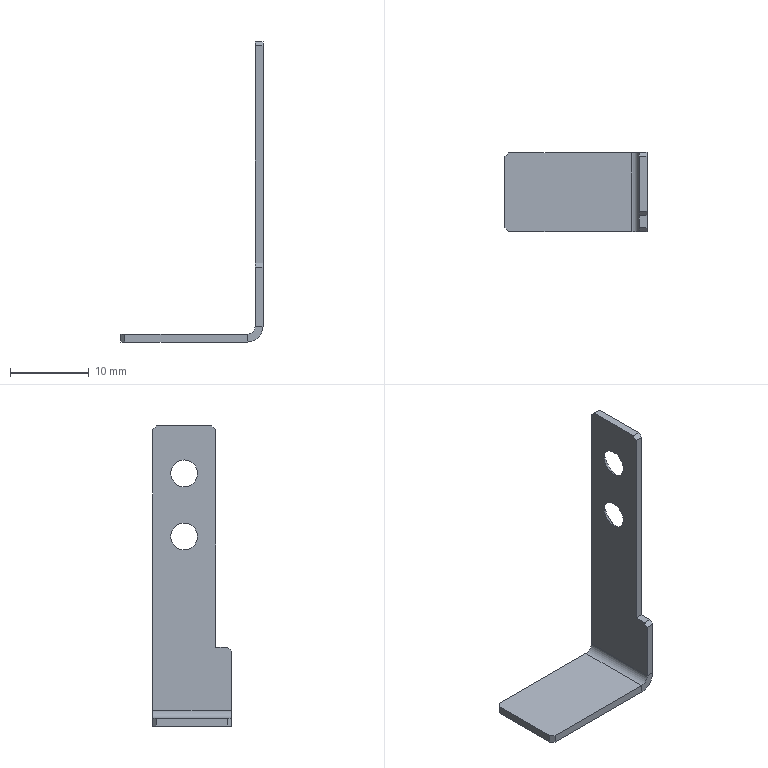Part | NX | features BREP 1 | 1 solid | 25 faces | box 18 x 10 x 38 mm | volume 456.003 mm3 | plane 19 | cone 4 | cylinder 2 | commonest cylinder face diameters 2 x1 4 x1
STEP:
#1=CARTESIAN_POINT('',(-1.,4.5,19.));
#2=VERTEX_POINT('',#1);
#3=CARTESIAN_POINT('',(-1.,5.,18.5));
#4=VERTEX_POINT('',#3);
#5=CARTESIAN_POINT('',(-1.,5.,18.5));
#6=DIRECTION('',(0.,0.7071,-0.7071));
#7=VECTOR('',#6,1000.);
#8=LINE('',#5,#7);
#9=EDGE_CURVE('',#2,#4,#8,.T.);
#10=ORIENTED_EDGE('',*,*,#9,.F.);
#11=CARTESIAN_POINT('',(0.,4.5,19.));
#12=VERTEX_POINT('',#11);
#13=CARTESIAN_POINT('',(-1.,4.5,19.));
#14=DIRECTION('',(-1.,0.,0.));
#15=VECTOR('',#14,1000.);
#16=LINE('',#13,#15);
#17=EDGE_CURVE('',#12,#2,#16,.T.);
#18=ORIENTED_EDGE('',*,*,#17,.F.);
#19=CARTESIAN_POINT('',(0.,5.,18.5));
#20=VERTEX_POINT('',#19);
#21=CARTESIAN_POINT('',(0.,11.75,11.75));
#22=DIRECTION('',(0.,-0.7071,0.7071));
#23=VECTOR('',#22,1000.);
#24=LINE('',#21,#23);
#25=EDGE_CURVE('',#20,#12,#24,.T.);
#26=ORIENTED_EDGE('',*,*,#25,.F.);
#27=CARTESIAN_POINT('',(-1.,5.,18.5));
#28=DIRECTION('',(1.,0.,0.));
#29=VECTOR('',#28,1000.);
#30=LINE('',#27,#29);
#31=EDGE_CURVE('',#4,#20,#30,.T.);
#32=ORIENTED_EDGE('',*,*,#31,.F.);
#33=EDGE_LOOP('',(#10,#18,#26,#32));
#34=FACE_BOUND('',#33,.T.);
#35=CARTESIAN_POINT('',(-1.,5.,18.5));
#36=DIRECTION('',(0.,-0.7071,-0.7071));
#37=DIRECTION('',(1.,0.,0.));
#38=AXIS2_PLACEMENT_3D('',#35,#36,#37);
#39=PLANE('',#38);
#40=ADVANCED_FACE('',(#34),#39,.F.);
#41=CARTESIAN_POINT('',(0.,-2.5,19.));
#42=VERTEX_POINT('',#41);
#43=CARTESIAN_POINT('',(0.,-3.,18.5));
#44=VERTEX_POINT('',#43);
#45=CARTESIAN_POINT('',(0.,-10.75,10.75));
#46=DIRECTION('',(0.,-0.7071,-0.7071));
#47=VECTOR('',#46,1000.);
#48=LINE('',#45,#47);
#49=EDGE_CURVE('',#42,#44,#48,.T.);
#50=ORIENTED_EDGE('',*,*,#49,.F.);
#51=CARTESIAN_POINT('',(-1.,-2.5,19.));
#52=VERTEX_POINT('',#51);
#53=CARTESIAN_POINT('',(0.,-2.5,19.));
#54=DIRECTION('',(1.,0.,0.));
#55=VECTOR('',#54,1000.);
#56=LINE('',#53,#55);
#57=EDGE_CURVE('',#52,#42,#56,.T.);
#58=ORIENTED_EDGE('',*,*,#57,.F.);
#59=CARTESIAN_POINT('',(-1.,-3.,18.5));
#60=VERTEX_POINT('',#59);
#61=CARTESIAN_POINT('',(-1.,-3.,18.5));
#62=DIRECTION('',(0.,0.7071,0.7071));
#63=VECTOR('',#62,1000.);
#64=LINE('',#61,#63);
#65=EDGE_CURVE('',#60,#52,#64,.T.);
#66=ORIENTED_EDGE('',*,*,#65,.F.);
#67=CARTESIAN_POINT('',(-1.,-3.,18.5));
#68=DIRECTION('',(-1.,0.,0.));
#69=VECTOR('',#68,1000.);
#70=LINE('',#67,#69);
#71=EDGE_CURVE('',#44,#60,#70,.T.);
#72=ORIENTED_EDGE('',*,*,#71,.F.);
#73=EDGE_LOOP('',(#50,#58,#66,#72));
#74=FACE_BOUND('',#73,.T.);
#75=CARTESIAN_POINT('',(-18.,-3.,18.5));
#76=DIRECTION('',(0.,-0.7071,0.7071));
#77=DIRECTION('',(1.,0.,0.));
#78=AXIS2_PLACEMENT_3D('',#75,#76,#77);
#79=PLANE('',#78);
#80=ADVANCED_FACE('',(#74),#79,.T.);
#81=CARTESIAN_POINT('',(-1.,-5.,-9.5));
#82=VERTEX_POINT('',#81);
#83=CARTESIAN_POINT('',(-1.,-4.5,-9.));
#84=VERTEX_POINT('',#83);
#85=CARTESIAN_POINT('',(-1.,-4.5,-9.));
#86=DIRECTION('',(0.,0.7071,0.7071));
#87=VECTOR('',#86,1000.);
#88=LINE('',#85,#87);
#89=EDGE_CURVE('',#82,#84,#88,.T.);
#90=ORIENTED_EDGE('',*,*,#89,.F.);
#91=CARTESIAN_POINT('',(0.,-5.,-9.5));
#92=VERTEX_POINT('',#91);
#93=CARTESIAN_POINT('',(-1.,-5.,-9.5));
#94=DIRECTION('',(-1.,0.,0.));
#95=VECTOR('',#94,1000.);
#96=LINE('',#93,#95);
#97=EDGE_CURVE('',#92,#82,#96,.T.);
#98=ORIENTED_EDGE('',*,*,#97,.F.);
#99=CARTESIAN_POINT('',(0.,-4.5,-9.));
#100=VERTEX_POINT('',#99);
#101=CARTESIAN_POINT('',(0.,2.25,-2.25));
#102=DIRECTION('',(0.,-0.7071,-0.7071));
#103=VECTOR('',#102,1000.);
#104=LINE('',#101,#103);
#105=EDGE_CURVE('',#100,#92,#104,.T.);
#106=ORIENTED_EDGE('',*,*,#105,.F.);
#107=CARTESIAN_POINT('',(0.,-4.5,-9.));
#108=DIRECTION('',(1.,0.,0.));
#109=VECTOR('',#108,1000.);
#110=LINE('',#107,#109);
#111=EDGE_CURVE('',#84,#100,#110,.T.);
#112=ORIENTED_EDGE('',*,*,#111,.F.);
#113=EDGE_LOOP('',(#90,#98,#106,#112));
#114=FACE_BOUND('',#113,.T.);
#115=CARTESIAN_POINT('',(-18.,-4.5,-9.));
#116=DIRECTION('',(0.,-0.7071,0.7071));
#117=DIRECTION('',(-1.,0.,0.));
#118=AXIS2_PLACEMENT_3D('',#115,#116,#117);
#119=PLANE('',#118);
#120=ADVANCED_FACE('',(#114),#119,.T.);
#121=CARTESIAN_POINT('',(-17.5,-5.,-19.));
#122=VERTEX_POINT('',#121);
#123=CARTESIAN_POINT('',(-18.,-4.5,-19.));
#124=VERTEX_POINT('',#123);
#125=CARTESIAN_POINT('',(-18.,-4.5,-19.));
#126=DIRECTION('',(-0.7071,0.7071,0.));
#127=VECTOR('',#126,1000.);
#128=LINE('',#125,#127);
#129=EDGE_CURVE('',#122,#124,#128,.T.);
#130=ORIENTED_EDGE('',*,*,#129,.F.);
#131=CARTESIAN_POINT('',(-17.5,-5.,-18.));
#132=VERTEX_POINT('',#131);
#133=CARTESIAN_POINT('',(-17.5,-5.,-19.));
#134=DIRECTION('',(0.,0.,-1.));
#135=VECTOR('',#134,1000.);
#136=LINE('',#133,#135);
#137=EDGE_CURVE('',#132,#122,#136,.T.);
#138=ORIENTED_EDGE('',*,*,#137,.F.);
#139=CARTESIAN_POINT('',(-18.,-4.5,-18.));
#140=VERTEX_POINT('',#139);
#141=CARTESIAN_POINT('',(-11.25,-11.25,-18.));
#142=DIRECTION('',(0.7071,-0.7071,0.));
#143=VECTOR('',#142,1000.);
#144=LINE('',#141,#143);
#145=EDGE_CURVE('',#140,#132,#144,.T.);
#146=ORIENTED_EDGE('',*,*,#145,.F.);
#147=CARTESIAN_POINT('',(-18.,-4.5,-19.));
#148=DIRECTION('',(0.,0.,1.));
#149=VECTOR('',#148,1000.);
#150=LINE('',#147,#149);
#151=EDGE_CURVE('',#124,#140,#150,.T.);
#152=ORIENTED_EDGE('',*,*,#151,.F.);
#153=EDGE_LOOP('',(#130,#138,#146,#152));
#154=FACE_BOUND('',#153,.T.);
#155=CARTESIAN_POINT('',(-18.,-4.5,-19.));
#156=DIRECTION('',(0.7071,0.7071,0.));
#157=DIRECTION('',(0.,0.,1.));
#158=AXIS2_PLACEMENT_3D('',#155,#156,#157);
#159=PLANE('',#158);
#160=ADVANCED_FACE('',(#154),#159,.F.);
#161=CARTESIAN_POINT('',(-18.,4.5,-19.));
#162=VERTEX_POINT('',#161);
#163=CARTESIAN_POINT('',(-17.5,5.,-19.));
#164=VERTEX_POINT('',#163);
#165=CARTESIAN_POINT('',(-17.5,5.,-19.));
#166=DIRECTION('',(0.7071,0.7071,0.));
#167=VECTOR('',#166,1000.);
#168=LINE('',#165,#167);
#169=EDGE_CURVE('',#162,#164,#168,.T.);
#170=ORIENTED_EDGE('',*,*,#169,.F.);
#171=CARTESIAN_POINT('',(-18.,4.5,-18.));
#172=VERTEX_POINT('',#171);
#173=CARTESIAN_POINT('',(-18.,4.5,-19.));
#174=DIRECTION('',(0.,0.,-1.));
#175=VECTOR('',#174,1000.);
#176=LINE('',#173,#175);
#177=EDGE_CURVE('',#172,#162,#176,.T.);
#178=ORIENTED_EDGE('',*,*,#177,.F.);
#179=CARTESIAN_POINT('',(-17.5,5.,-18.));
#180=VERTEX_POINT('',#179);
#181=CARTESIAN_POINT('',(-11.25,11.25,-18.));
#182=DIRECTION('',(-0.7071,-0.7071,0.));
#183=VECTOR('',#182,1000.);
#184=LINE('',#181,#183);
#185=EDGE_CURVE('',#180,#172,#184,.T.);
#186=ORIENTED_EDGE('',*,*,#185,.F.);
#187=CARTESIAN_POINT('',(-17.5,5.,-19.));
#188=DIRECTION('',(0.,0.,1.));
#189=VECTOR('',#188,1000.);
#190=LINE('',#187,#189);
#191=EDGE_CURVE('',#164,#180,#190,.T.);
#192=ORIENTED_EDGE('',*,*,#191,.F.);
#193=EDGE_LOOP('',(#170,#178,#186,#192));
#194=FACE_BOUND('',#193,.T.);
#195=CARTESIAN_POINT('',(-17.5,5.,-19.));
#196=DIRECTION('',(0.7071,-0.7071,0.));
#197=DIRECTION('',(0.,0.,1.));
#198=AXIS2_PLACEMENT_3D('',#195,#196,#197);
#199=PLANE('',#198);
#200=ADVANCED_FACE('',(#194),#199,.F.);
#201=CARTESIAN_POINT('',(-1.,1.,14.7));
#202=VERTEX_POINT('',#201);
#203=CARTESIAN_POINT('',(0.,1.,15.7));
#204=VERTEX_POINT('',#203);
#205=CARTESIAN_POINT('',(-1.,1.,14.7));
#206=DIRECTION('',(0.7071,0.,0.7071));
#207=VECTOR('',#206,1000.);
#208=LINE('',#205,#207);
#209=EDGE_CURVE('',#202,#204,#208,.T.);
#210=ORIENTED_EDGE('',*,*,#209,.F.);
#211=CARTESIAN_POINT('',(-1.,1.,11.3));
#212=VERTEX_POINT('',#211);
#213=CARTESIAN_POINT('',(-1.,1.,13.));
#214=DIRECTION('',(1.,0.,0.));
#215=DIRECTION('',(0.,0.,-1.));
#216=AXIS2_PLACEMENT_3D('',#213,#214,#215);
#217=CIRCLE('',#216,1.7);
#218=EDGE_CURVE('',#212,#202,#217,.T.);
#219=ORIENTED_EDGE('',*,*,#218,.F.);
#220=CARTESIAN_POINT('',(0.,1.,10.3));
#221=VERTEX_POINT('',#220);
#222=CARTESIAN_POINT('',(-1.,1.,11.3));
#223=DIRECTION('',(0.7071,0.,-0.7071));
#224=VECTOR('',#223,1000.);
#225=LINE('',#222,#224);
#226=EDGE_CURVE('',#212,#221,#225,.T.);
#227=ORIENTED_EDGE('',*,*,#226,.T.);
#228=CARTESIAN_POINT('',(0.,1.,13.));
#229=DIRECTION('',(-1.,0.,0.));
#230=DIRECTION('',(0.,0.,-1.));
#231=AXIS2_PLACEMENT_3D('',#228,#229,#230);
#232=CIRCLE('',#231,2.7);
#233=EDGE_CURVE('',#204,#221,#232,.T.);
#234=ORIENTED_EDGE('',*,*,#233,.F.);
#235=EDGE_LOOP('',(#210,#219,#227,#234));
#236=FACE_BOUND('',#235,.T.);
#237=CARTESIAN_POINT('',(-1.,1.,13.));
#238=DIRECTION('',(1.,0.,0.));
#239=DIRECTION('',(0.,0.,-1.));
#240=AXIS2_PLACEMENT_3D('',#237,#238,#239);
#241=CONICAL_SURFACE('',#240,1.7,0.7854);
#242=ADVANCED_FACE('',(#236),#241,.F.);
#243=CARTESIAN_POINT('',(-1.,1.,6.7));
#244=VERTEX_POINT('',#243);
#245=CARTESIAN_POINT('',(0.,1.,7.7));
#246=VERTEX_POINT('',#245);
#247=CARTESIAN_POINT('',(-1.,1.,6.7));
#248=DIRECTION('',(0.7071,0.,0.7071));
#249=VECTOR('',#248,1000.);
#250=LINE('',#247,#249);
#251=EDGE_CURVE('',#244,#246,#250,.T.);
#252=ORIENTED_EDGE('',*,*,#251,.F.);
#253=CARTESIAN_POINT('',(-1.,1.,3.3));
#254=VERTEX_POINT('',#253);
#255=CARTESIAN_POINT('',(-1.,1.,5.));
#256=DIRECTION('',(1.,0.,0.));
#257=DIRECTION('',(0.,0.,-1.));
#258=AXIS2_PLACEMENT_3D('',#255,#256,#257);
#259=CIRCLE('',#258,1.7);
#260=EDGE_CURVE('',#254,#244,#259,.T.);
#261=ORIENTED_EDGE('',*,*,#260,.F.);
#262=CARTESIAN_POINT('',(0.,1.,2.3));
#263=VERTEX_POINT('',#262);
#264=CARTESIAN_POINT('',(-1.,1.,3.3));
#265=DIRECTION('',(0.7071,0.,-0.7071));
#266=VECTOR('',#265,1000.);
#267=LINE('',#264,#266);
#268=EDGE_CURVE('',#254,#263,#267,.T.);
#269=ORIENTED_EDGE('',*,*,#268,.T.);
#270=CARTESIAN_POINT('',(0.,1.,5.));
#271=DIRECTION('',(-1.,0.,0.));
#272=DIRECTION('',(0.,0.,-1.));
#273=AXIS2_PLACEMENT_3D('',#270,#271,#272);
#274=CIRCLE('',#273,2.7);
#275=EDGE_CURVE('',#246,#263,#274,.T.);
#276=ORIENTED_EDGE('',*,*,#275,.F.);
#277=EDGE_LOOP('',(#252,#261,#269,#276));
#278=FACE_BOUND('',#277,.T.);
#279=CARTESIAN_POINT('',(-1.,1.,5.));
#280=DIRECTION('',(1.,0.,0.));
#281=DIRECTION('',(0.,0.,-1.));
#282=AXIS2_PLACEMENT_3D('',#279,#280,#281);
#283=CONICAL_SURFACE('',#282,1.7,0.7854);
#284=ADVANCED_FACE('',(#278),#283,.F.);
#285=CARTESIAN_POINT('',(0.,-3.,-9.));
#286=VERTEX_POINT('',#285);
#287=CARTESIAN_POINT('',(0.,-3.,-9.));
#288=DIRECTION('',(0.,0.,1.));
#289=VECTOR('',#288,1000.);
#290=LINE('',#287,#289);
#291=EDGE_CURVE('',#286,#44,#290,.T.);
#292=ORIENTED_EDGE('',*,*,#291,.T.);
#293=ORIENTED_EDGE('',*,*,#71,.T.);
#294=CARTESIAN_POINT('',(-1.,-3.,-9.));
#295=VERTEX_POINT('',#294);
#296=CARTESIAN_POINT('',(-1.,-3.,0.));
#297=DIRECTION('',(0.,0.,1.));
#298=VECTOR('',#297,1000.);
#299=LINE('',#296,#298);
#300=EDGE_CURVE('',#295,#60,#299,.T.);
#301=ORIENTED_EDGE('',*,*,#300,.F.);
#302=CARTESIAN_POINT('',(-18.,-3.,-9.));
#303=DIRECTION('',(1.,0.,0.));
#304=VECTOR('',#303,1000.);
#305=LINE('',#302,#304);
#306=EDGE_CURVE('',#295,#286,#305,.T.);
#307=ORIENTED_EDGE('',*,*,#306,.T.);
#308=EDGE_LOOP('',(#292,#293,#301,#307));
#309=FACE_BOUND('',#308,.T.);
#310=CARTESIAN_POINT('',(-18.,-3.,-9.));
#311=DIRECTION('',(0.,1.,0.));
#312=DIRECTION('',(0.,0.,1.));
#313=AXIS2_PLACEMENT_3D('',#310,#311,#312);
#314=PLANE('',#313);
#315=ADVANCED_FACE('',(#309),#314,.F.);
#316=CARTESIAN_POINT('',(-1.,0.,-9.));
#317=DIRECTION('',(0.,1.,0.));
#318=VECTOR('',#317,1000.);
#319=LINE('',#316,#318);
#320=EDGE_CURVE('',#84,#295,#319,.T.);
#321=ORIENTED_EDGE('',*,*,#320,.F.);
#322=ORIENTED_EDGE('',*,*,#111,.T.);
#323=CARTESIAN_POINT('',(0.,-3.,-9.));
#324=DIRECTION('',(0.,1.,0.));
#325=VECTOR('',#324,1000.);
#326=LINE('',#323,#325);
#327=EDGE_CURVE('',#100,#286,#326,.T.);
#328=ORIENTED_EDGE('',*,*,#327,.T.);
#329=ORIENTED_EDGE('',*,*,#306,.F.);
#330=EDGE_LOOP('',(#321,#322,#328,#329));
#331=FACE_BOUND('',#330,.T.);
#332=CARTESIAN_POINT('',(-18.,-3.,-9.));
#333=DIRECTION('',(0.,0.,-1.));
#334=DIRECTION('',(0.,1.,0.));
#335=AXIS2_PLACEMENT_3D('',#332,#333,#334);
#336=PLANE('',#335);
#337=ADVANCED_FACE('',(#331),#336,.F.);
#338=CARTESIAN_POINT('',(-18.,5.,-18.));
#339=DIRECTION('',(0.,1.,0.));
#340=VECTOR('',#339,1000.);
#341=LINE('',#338,#340);
#342=EDGE_CURVE('',#140,#172,#341,.T.);
#343=ORIENTED_EDGE('',*,*,#342,.T.);
#344=ORIENTED_EDGE('',*,*,#177,.T.);
#345=CARTESIAN_POINT('',(-18.,0.,-19.));
#346=DIRECTION('',(0.,1.,0.));
#347=VECTOR('',#346,1000.);
#348=LINE('',#345,#347);
#349=EDGE_CURVE('',#124,#162,#348,.T.);
#350=ORIENTED_EDGE('',*,*,#349,.F.);
#351=ORIENTED_EDGE('',*,*,#151,.T.);
#352=EDGE_LOOP('',(#343,#344,#350,#351));
#353=FACE_BOUND('',#352,.T.);
#354=CARTESIAN_POINT('',(-18.,5.,-19.));
#355=DIRECTION('',(1.,0.,0.));
#356=DIRECTION('',(0.,0.,-1.));
#357=AXIS2_PLACEMENT_3D('',#354,#355,#356);
#358=PLANE('',#357);
#359=ADVANCED_FACE('',(#353),#358,.F.);
#360=CARTESIAN_POINT('',(-2.,5.,-18.));
#361=VERTEX_POINT('',#360);
#362=CARTESIAN_POINT('',(-1.,5.,-18.));
#363=DIRECTION('',(1.,0.,0.));
#364=VECTOR('',#363,1000.);
#365=LINE('',#362,#364);
#366=EDGE_CURVE('',#180,#361,#365,.T.);
#367=ORIENTED_EDGE('',*,*,#366,.F.);
#368=ORIENTED_EDGE('',*,*,#185,.T.);
#369=ORIENTED_EDGE('',*,*,#342,.F.);
#370=ORIENTED_EDGE('',*,*,#145,.T.);
#371=CARTESIAN_POINT('',(-2.,-5.,-18.));
#372=VERTEX_POINT('',#371);
#373=CARTESIAN_POINT('',(-18.,-5.,-18.));
#374=DIRECTION('',(-1.,0.,0.));
#375=VECTOR('',#374,1000.);
#376=LINE('',#373,#375);
#377=EDGE_CURVE('',#372,#132,#376,.T.);
#378=ORIENTED_EDGE('',*,*,#377,.F.);
#379=CARTESIAN_POINT('',(-2.,5.,-18.));
#380=DIRECTION('',(0.,-1.,0.));
#381=VECTOR('',#380,1000.);
#382=LINE('',#379,#381);
#383=EDGE_CURVE('',#361,#372,#382,.T.);
#384=ORIENTED_EDGE('',*,*,#383,.F.);
#385=EDGE_LOOP('',(#367,#368,#369,#370,#378,#384));
#386=FACE_BOUND('',#385,.T.);
#387=CARTESIAN_POINT('',(0.,0.,-18.));
#388=DIRECTION('',(0.,0.,1.));
#389=DIRECTION('',(1.,0.,0.));
#390=AXIS2_PLACEMENT_3D('',#387,#388,#389);
#391=PLANE('',#390);
#392=ADVANCED_FACE('',(#386),#391,.T.);
#393=ORIENTED_EDGE('',*,*,#349,.T.);
#394=ORIENTED_EDGE('',*,*,#169,.T.);
#395=CARTESIAN_POINT('',(-2.,5.,-19.));
#396=VERTEX_POINT('',#395);
#397=CARTESIAN_POINT('',(0.,5.,-19.));
#398=DIRECTION('',(1.,0.,0.));
#399=VECTOR('',#398,1000.);
#400=LINE('',#397,#399);
#401=EDGE_CURVE('',#164,#396,#400,.T.);
#402=ORIENTED_EDGE('',*,*,#401,.T.);
#403=CARTESIAN_POINT('',(-2.,-5.,-19.));
#404=VERTEX_POINT('',#403);
#405=CARTESIAN_POINT('',(-2.,5.,-19.));
#406=DIRECTION('',(0.,1.,0.));
#407=VECTOR('',#406,1000.);
#408=LINE('',#405,#407);
#409=EDGE_CURVE('',#404,#396,#408,.T.);
#410=ORIENTED_EDGE('',*,*,#409,.F.);
#411=CARTESIAN_POINT('',(0.,-5.,-19.));
#412=DIRECTION('',(-1.,0.,0.));
#413=VECTOR('',#412,1000.);
#414=LINE('',#411,#413);
#415=EDGE_CURVE('',#404,#122,#414,.T.);
#416=ORIENTED_EDGE('',*,*,#415,.T.);
#417=ORIENTED_EDGE('',*,*,#129,.T.);
#418=EDGE_LOOP('',(#393,#394,#402,#410,#416,#417));
#419=FACE_BOUND('',#418,.T.);
#420=CARTESIAN_POINT('',(0.,0.,-19.));
#421=DIRECTION('',(0.,0.,1.));
#422=DIRECTION('',(1.,0.,0.));
#423=AXIS2_PLACEMENT_3D('',#420,#421,#422);
#424=PLANE('',#423);
#425=ADVANCED_FACE('',(#419),#424,.F.);
#426=ORIENTED_EDGE('',*,*,#401,.F.);
#427=ORIENTED_EDGE('',*,*,#191,.T.);
#428=ORIENTED_EDGE('',*,*,#366,.T.);
#429=CARTESIAN_POINT('',(-2.,5.,-19.));
#430=DIRECTION('',(0.,0.,-1.));
#431=VECTOR('',#430,1000.);
#432=LINE('',#429,#431);
#433=EDGE_CURVE('',#361,#396,#432,.T.);
#434=ORIENTED_EDGE('',*,*,#433,.T.);
#435=EDGE_LOOP('',(#426,#427,#428,#434));
#436=FACE_BOUND('',#435,.T.);
#437=CARTESIAN_POINT('',(-1.,5.,-19.));
#438=DIRECTION('',(0.,-1.,0.));
#439=DIRECTION('',(0.,0.,-1.));
#440=AXIS2_PLACEMENT_3D('',#437,#438,#439);
#441=PLANE('',#440);
#442=ADVANCED_FACE('',(#436),#441,.F.);
#443=ORIENTED_EDGE('',*,*,#377,.T.);
#444=ORIENTED_EDGE('',*,*,#137,.T.);
#445=ORIENTED_EDGE('',*,*,#415,.F.);
#446=CARTESIAN_POINT('',(-2.,-5.,-18.));
#447=DIRECTION('',(0.,0.,-1.));
#448=VECTOR('',#447,1000.);
#449=LINE('',#446,#448);
#450=EDGE_CURVE('',#372,#404,#449,.T.);
#451=ORIENTED_EDGE('',*,*,#450,.F.);
#452=EDGE_LOOP('',(#443,#444,#445,#451));
#453=FACE_BOUND('',#452,.T.);
#454=CARTESIAN_POINT('',(-18.,-5.,-19.));
#455=DIRECTION('',(0.,1.,0.));
#456=DIRECTION('',(-1.,0.,0.));
#457=AXIS2_PLACEMENT_3D('',#454,#455,#456);
#458=PLANE('',#457);
#459=ADVANCED_FACE('',(#453),#458,.F.);
#460=CARTESIAN_POINT('',(-1.,-5.,-17.));
#461=VERTEX_POINT('',#460);
#462=CARTESIAN_POINT('',(-1.,5.,-17.));
#463=VERTEX_POINT('',#462);
#464=CARTESIAN_POINT('',(-1.,-5.,-17.));
#465=DIRECTION('',(0.,1.,0.));
#466=VECTOR('',#465,1000.);
#467=LINE('',#464,#466);
#468=EDGE_CURVE('',#461,#463,#467,.T.);
#469=ORIENTED_EDGE('',*,*,#468,.T.);
#470=CARTESIAN_POINT('',(-2.,5.,-17.));
#471=DIRECTION('',(0.,1.,0.));
#472=DIRECTION('',(0.,0.,-1.));
#473=AXIS2_PLACEMENT_3D('',#470,#471,#472);
#474=CIRCLE('',#473,1.);
#475=EDGE_CURVE('',#463,#361,#474,.T.);
#476=ORIENTED_EDGE('',*,*,#475,.T.);
#477=ORIENTED_EDGE('',*,*,#383,.T.);
#478=CARTESIAN_POINT('',(-2.,-5.,-17.));
#479=DIRECTION('',(0.,-1.,0.));
#480=DIRECTION('',(0.,0.,-1.));
#481=AXIS2_PLACEMENT_3D('',#478,#479,#480);
#482=CIRCLE('',#481,1.);
#483=EDGE_CURVE('',#372,#461,#482,.T.);
#484=ORIENTED_EDGE('',*,*,#483,.T.);
#485=EDGE_LOOP('',(#469,#476,#477,#484));
#486=FACE_BOUND('',#485,.T.);
#487=CARTESIAN_POINT('',(-2.,-5.,-17.));
#488=DIRECTION('',(0.,-1.,0.));
#489=DIRECTION('',(0.,0.,-1.));
#490=AXIS2_PLACEMENT_3D('',#487,#488,#489);
#491=CYLINDRICAL_SURFACE('',#490,1.);
#492=ADVANCED_FACE('',(#486),#491,.F.);
#493=CARTESIAN_POINT('',(0.,-5.,-17.));
#494=VERTEX_POINT('',#493);
#495=CARTESIAN_POINT('',(0.,5.,-17.));
#496=VERTEX_POINT('',#495);
#497=CARTESIAN_POINT('',(0.,-5.,-17.));
#498=DIRECTION('',(0.,1.,0.));
#499=VECTOR('',#498,1000.);
#500=LINE('',#497,#499);
#501=EDGE_CURVE('',#494,#496,#500,.T.);
#502=ORIENTED_EDGE('',*,*,#501,.F.);
#503=CARTESIAN_POINT('',(-2.,-5.,-17.));
#504=DIRECTION('',(0.,-1.,0.));
#505=DIRECTION('',(0.,0.,-1.));
#506=AXIS2_PLACEMENT_3D('',#503,#504,#505);
#507=CIRCLE('',#506,2.);
#508=EDGE_CURVE('',#404,#494,#507,.T.);
#509=ORIENTED_EDGE('',*,*,#508,.F.);
#510=ORIENTED_EDGE('',*,*,#409,.T.);
#511=CARTESIAN_POINT('',(-2.,5.,-17.));
#512=DIRECTION('',(0.,1.,0.));
#513=DIRECTION('',(0.,0.,-1.));
#514=AXIS2_PLACEMENT_3D('',#511,#512,#513);
#515=CIRCLE('',#514,2.);
#516=EDGE_CURVE('',#496,#396,#515,.T.);
#517=ORIENTED_EDGE('',*,*,#516,.F.);
#518=EDGE_LOOP('',(#502,#509,#510,#517));
#519=FACE_BOUND('',#518,.T.);
#520=CARTESIAN_POINT('',(-2.,-5.,-17.));
#521=DIRECTION('',(0.,-1.,0.));
#522=DIRECTION('',(0.,0.,-1.));
#523=AXIS2_PLACEMENT_3D('',#520,#521,#522);
#524=CYLINDRICAL_SURFACE('',#523,2.);
#525=ADVANCED_FACE('',(#519),#524,.T.);
#526=ORIENTED_EDGE('',*,*,#483,.F.);
#527=ORIENTED_EDGE('',*,*,#450,.T.);
#528=ORIENTED_EDGE('',*,*,#508,.T.);
#529=CARTESIAN_POINT('',(-1.,-5.,-17.));
#530=DIRECTION('',(1.,0.,0.));
#531=VECTOR('',#530,1000.);
#532=LINE('',#529,#531);
#533=EDGE_CURVE('',#461,#494,#532,.T.);
#534=ORIENTED_EDGE('',*,*,#533,.F.);
#535=EDGE_LOOP('',(#526,#527,#528,#534));
#536=FACE_BOUND('',#535,.T.);
#537=CARTESIAN_POINT('',(-2.,-5.,-17.));
#538=DIRECTION('',(0.,1.,0.));
#539=DIRECTION('',(0.,0.,1.));
#540=AXIS2_PLACEMENT_3D('',#537,#538,#539);
#541=PLANE('',#540);
#542=ADVANCED_FACE('',(#536),#541,.F.);
#543=ORIENTED_EDGE('',*,*,#433,.F.);
#544=ORIENTED_EDGE('',*,*,#475,.F.);
#545=CARTESIAN_POINT('',(-1.,5.,-17.));
#546=DIRECTION('',(1.,0.,0.));
#547=VECTOR('',#546,1000.);
#548=LINE('',#545,#547);
#549=EDGE_CURVE('',#463,#496,#548,.T.);
#550=ORIENTED_EDGE('',*,*,#549,.T.);
#551=ORIENTED_EDGE('',*,*,#516,.T.);
#552=EDGE_LOOP('',(#543,#544,#550,#551));
#553=FACE_BOUND('',#552,.T.);
#554=CARTESIAN_POINT('',(-2.,5.,-17.));
#555=DIRECTION('',(0.,1.,0.));
#556=DIRECTION('',(0.,0.,1.));
#557=AXIS2_PLACEMENT_3D('',#554,#555,#556);
#558=PLANE('',#557);
#559=ADVANCED_FACE('',(#553),#558,.T.);
#560=CARTESIAN_POINT('',(-1.,5.,19.));
#561=DIRECTION('',(0.,0.,1.));
#562=VECTOR('',#561,1000.);
#563=LINE('',#560,#562);
#564=EDGE_CURVE('',#463,#4,#563,.T.);
#565=ORIENTED_EDGE('',*,*,#564,.T.);
#566=ORIENTED_EDGE('',*,*,#31,.T.);
#567=CARTESIAN_POINT('',(0.,5.,19.));
#568=DIRECTION('',(0.,0.,1.));
#569=VECTOR('',#568,1000.);
#570=LINE('',#567,#569);
#571=EDGE_CURVE('',#496,#20,#570,.T.);
#572=ORIENTED_EDGE('',*,*,#571,.F.);
#573=ORIENTED_EDGE('',*,*,#549,.F.);
#574=EDGE_LOOP('',(#565,#566,#572,#573));
#575=FACE_BOUND('',#574,.T.);
#576=CARTESIAN_POINT('',(-1.,5.,19.));
#577=DIRECTION('',(0.,1.,0.));
#578=DIRECTION('',(0.,0.,1.));
#579=AXIS2_PLACEMENT_3D('',#576,#577,#578);
#580=PLANE('',#579);
#581=ADVANCED_FACE('',(#575),#580,.T.);
#582=CARTESIAN_POINT('',(-1.,5.,19.));
#583=DIRECTION('',(0.,-1.,0.));
#584=VECTOR('',#583,1000.);
#585=LINE('',#582,#584);
#586=EDGE_CURVE('',#2,#52,#585,.T.);
#587=ORIENTED_EDGE('',*,*,#586,.T.);
#588=ORIENTED_EDGE('',*,*,#57,.T.);
#589=CARTESIAN_POINT('',(0.,5.,19.));
#590=DIRECTION('',(0.,-1.,0.));
#591=VECTOR('',#590,1000.);
#592=LINE('',#589,#591);
#593=EDGE_CURVE('',#12,#42,#592,.T.);
#594=ORIENTED_EDGE('',*,*,#593,.F.);
#595=ORIENTED_EDGE('',*,*,#17,.T.);
#596=EDGE_LOOP('',(#587,#588,#594,#595));
#597=FACE_BOUND('',#596,.T.);
#598=CARTESIAN_POINT('',(-1.,5.,19.));
#599=DIRECTION('',(0.,0.,1.));
#600=DIRECTION('',(1.,0.,0.));
#601=AXIS2_PLACEMENT_3D('',#598,#599,#600);
#602=PLANE('',#601);
#603=ADVANCED_FACE('',(#597),#602,.T.);
#604=ORIENTED_EDGE('',*,*,#327,.F.);
#605=ORIENTED_EDGE('',*,*,#105,.T.);
#606=CARTESIAN_POINT('',(0.,-5.,19.));
#607=DIRECTION('',(0.,0.,-1.));
#608=VECTOR('',#607,1000.);
#609=LINE('',#606,#608);
#610=EDGE_CURVE('',#92,#494,#609,.T.);
#611=ORIENTED_EDGE('',*,*,#610,.T.);
#612=ORIENTED_EDGE('',*,*,#501,.T.);
#613=ORIENTED_EDGE('',*,*,#571,.T.);
#614=ORIENTED_EDGE('',*,*,#25,.T.);
#615=ORIENTED_EDGE('',*,*,#593,.T.);
#616=ORIENTED_EDGE('',*,*,#49,.T.);
#617=ORIENTED_EDGE('',*,*,#291,.F.);
#618=EDGE_LOOP('',(#604,#605,#611,#612,#613,#614,#615,#616,#617));
#619=FACE_BOUND('',#618,.T.);
#620=CARTESIAN_POINT('',(0.,1.,13.));
#621=DIRECTION('',(-1.,0.,0.));
#622=DIRECTION('',(0.,0.,-1.));
#623=AXIS2_PLACEMENT_3D('',#620,#621,#622);
#624=CIRCLE('',#623,2.7);
#625=EDGE_CURVE('',#221,#204,#624,.T.);
#626=ORIENTED_EDGE('',*,*,#625,.T.);
#627=ORIENTED_EDGE('',*,*,#233,.T.);
#628=EDGE_LOOP('',(#626,#627));
#629=FACE_BOUND('',#628,.T.);
#630=CARTESIAN_POINT('',(0.,1.,5.));
#631=DIRECTION('',(-1.,0.,0.));
#632=DIRECTION('',(0.,0.,-1.));
#633=AXIS2_PLACEMENT_3D('',#630,#631,#632);
#634=CIRCLE('',#633,2.7);
#635=EDGE_CURVE('',#263,#246,#634,.T.);
#636=ORIENTED_EDGE('',*,*,#635,.T.);
#637=ORIENTED_EDGE('',*,*,#275,.T.);
#638=EDGE_LOOP('',(#636,#637));
#639=FACE_BOUND('',#638,.T.);
#640=CARTESIAN_POINT('',(0.,0.,0.));
#641=DIRECTION('',(1.,0.,0.));
#642=DIRECTION('',(0.,0.,-1.));
#643=AXIS2_PLACEMENT_3D('',#640,#641,#642);
#644=PLANE('',#643);
#645=ADVANCED_FACE('',(#619,#629,#639),#644,.T.);
#646=CARTESIAN_POINT('',(-1.,-5.,19.));
#647=DIRECTION('',(0.,0.,-1.));
#648=VECTOR('',#647,1000.);
#649=LINE('',#646,#648);
#650=EDGE_CURVE('',#82,#461,#649,.T.);
#651=ORIENTED_EDGE('',*,*,#650,.F.);
#652=ORIENTED_EDGE('',*,*,#89,.T.);
#653=ORIENTED_EDGE('',*,*,#320,.T.);
#654=ORIENTED_EDGE('',*,*,#300,.T.);
#655=ORIENTED_EDGE('',*,*,#65,.T.);
#656=ORIENTED_EDGE('',*,*,#586,.F.);
#657=ORIENTED_EDGE('',*,*,#9,.T.);
#658=ORIENTED_EDGE('',*,*,#564,.F.);
#659=ORIENTED_EDGE('',*,*,#468,.F.);
#660=EDGE_LOOP('',(#651,#652,#653,#654,#655,#656,#657,#658,#659));
#661=FACE_BOUND('',#660,.T.);
#662=ORIENTED_EDGE('',*,*,#260,.T.);
#663=CARTESIAN_POINT('',(-1.,1.,5.));
#664=DIRECTION('',(1.,0.,0.));
#665=DIRECTION('',(0.,0.,-1.));
#666=AXIS2_PLACEMENT_3D('',#663,#664,#665);
#667=CIRCLE('',#666,1.7);
#668=EDGE_CURVE('',#244,#254,#667,.T.);
#669=ORIENTED_EDGE('',*,*,#668,.T.);
#670=EDGE_LOOP('',(#662,#669));
#671=FACE_BOUND('',#670,.T.);
#672=ORIENTED_EDGE('',*,*,#218,.T.);
#673=CARTESIAN_POINT('',(-1.,1.,13.));
#674=DIRECTION('',(1.,0.,0.));
#675=DIRECTION('',(0.,0.,-1.));
#676=AXIS2_PLACEMENT_3D('',#673,#674,#675);
#677=CIRCLE('',#676,1.7);
#678=EDGE_CURVE('',#202,#212,#677,.T.);
#679=ORIENTED_EDGE('',*,*,#678,.T.);
#680=EDGE_LOOP('',(#672,#679));
#681=FACE_BOUND('',#680,.T.);
#682=CARTESIAN_POINT('',(-1.,0.,0.));
#683=DIRECTION('',(1.,0.,0.));
#684=DIRECTION('',(0.,0.,-1.));
#685=AXIS2_PLACEMENT_3D('',#682,#683,#684);
#686=PLANE('',#685);
#687=ADVANCED_FACE('',(#661,#671,#681),#686,.F.);
#688=ORIENTED_EDGE('',*,*,#610,.F.);
#689=ORIENTED_EDGE('',*,*,#97,.T.);
#690=ORIENTED_EDGE('',*,*,#650,.T.);
#691=ORIENTED_EDGE('',*,*,#533,.T.);
#692=EDGE_LOOP('',(#688,#689,#690,#691));
#693=FACE_BOUND('',#692,.T.);
#694=CARTESIAN_POINT('',(-1.,-5.,19.));
#695=DIRECTION('',(0.,-1.,0.));
#696=DIRECTION('',(0.,0.,-1.));
#697=AXIS2_PLACEMENT_3D('',#694,#695,#696);
#698=PLANE('',#697);
#699=ADVANCED_FACE('',(#693),#698,.T.);
#700=ORIENTED_EDGE('',*,*,#668,.F.);
#701=ORIENTED_EDGE('',*,*,#251,.T.);
#702=ORIENTED_EDGE('',*,*,#635,.F.);
#703=ORIENTED_EDGE('',*,*,#268,.F.);
#704=EDGE_LOOP('',(#700,#701,#702,#703));
#705=FACE_BOUND('',#704,.T.);
#706=CARTESIAN_POINT('',(-1.,1.,5.));
#707=DIRECTION('',(1.,0.,0.));
#708=DIRECTION('',(0.,0.,-1.));
#709=AXIS2_PLACEMENT_3D('',#706,#707,#708);
#710=CONICAL_SURFACE('',#709,1.7,0.7854);
#711=ADVANCED_FACE('',(#705),#710,.F.);
#712=ORIENTED_EDGE('',*,*,#678,.F.);
#713=ORIENTED_EDGE('',*,*,#209,.T.);
#714=ORIENTED_EDGE('',*,*,#625,.F.);
#715=ORIENTED_EDGE('',*,*,#226,.F.);
#716=EDGE_LOOP('',(#712,#713,#714,#715));
#717=FACE_BOUND('',#716,.T.);
#718=CARTESIAN_POINT('',(-1.,1.,13.));
#719=DIRECTION('',(1.,0.,0.));
#720=DIRECTION('',(0.,0.,-1.));
#721=AXIS2_PLACEMENT_3D('',#718,#719,#720);
#722=CONICAL_SURFACE('',#721,1.7,0.7854);
#723=ADVANCED_FACE('',(#717),#722,.F.);
#724=CLOSED_SHELL('',(#40,#80,#120,#160,#200,#242,#284,#315,#337,#359,#392,#425,#442,#459,#492,#525,#542,#559,#581,#603,#645,#687,#699,#711,#723));
#725=MANIFOLD_SOLID_BREP('',#724);
#726=(LENGTH_UNIT()NAMED_UNIT(*)SI_UNIT(.MILLI.,.METRE.));
#727=UNCERTAINTY_MEASURE_WITH_UNIT(LENGTH_MEASURE(0.00001),#726,'','');
#728=(NAMED_UNIT(*)PLANE_ANGLE_UNIT()SI_UNIT($,.RADIAN.));
#729=(NAMED_UNIT(*)SI_UNIT($,.STERADIAN.)SOLID_ANGLE_UNIT());
#730=(GEOMETRIC_REPRESENTATION_CONTEXT(3)GLOBAL_UNCERTAINTY_ASSIGNED_CONTEXT((#727))GLOBAL_UNIT_ASSIGNED_CONTEXT((#726,#728,#729))REPRESENTATION_CONTEXT('',''));
#731=ADVANCED_BREP_SHAPE_REPRESENTATION('',(#725),#730);